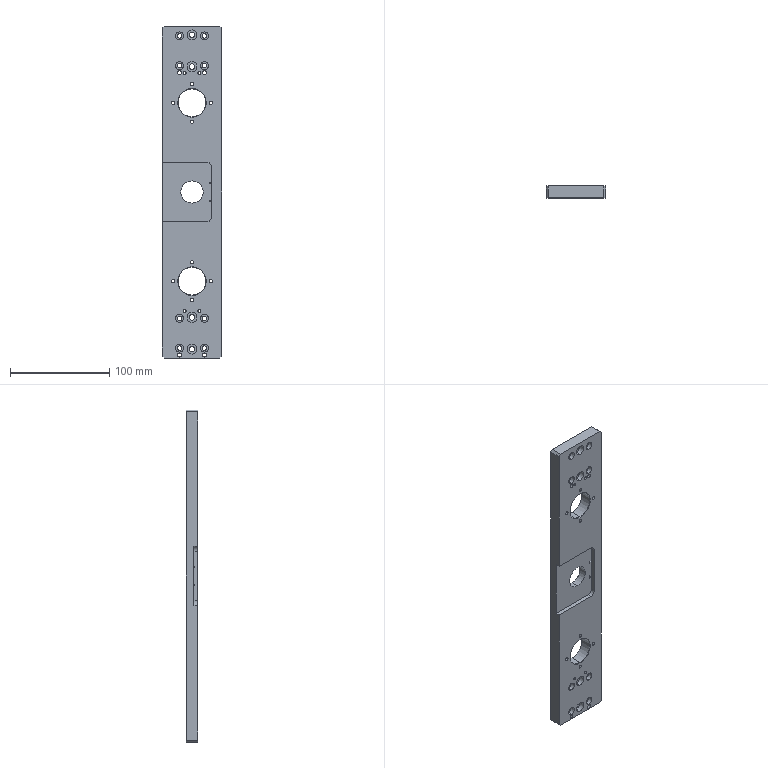Part | STEP file | PN_0025 | 1 solid | 132 faces | box 60 x 12 x 335 mm | volume 203956 mm3 | cylinder 92 | plane 26 | cone 14 | commonest cylinder face diameters 3.3 x16 4.5 x16 8 x16 10 x10 3 x8 4 x8